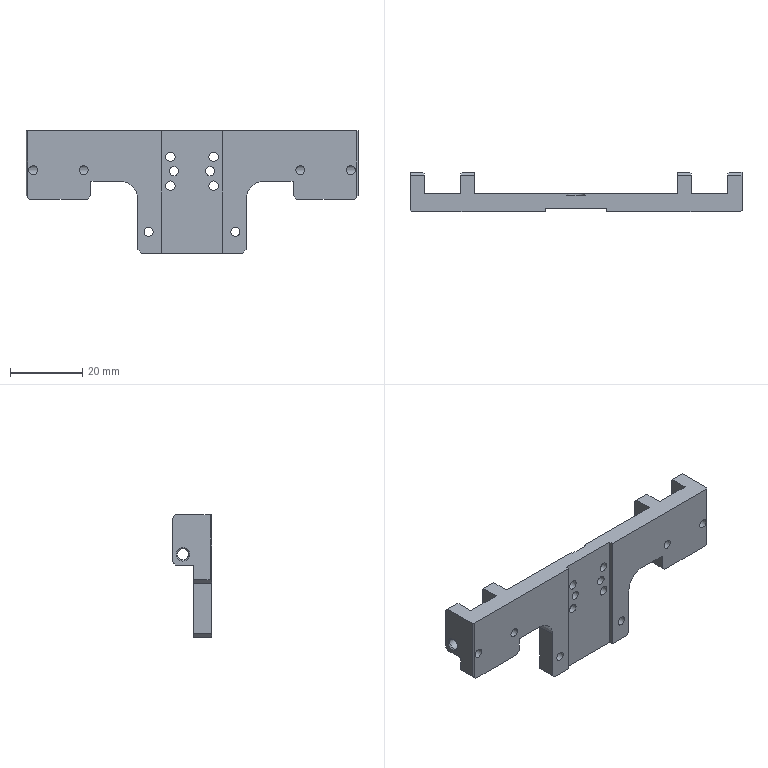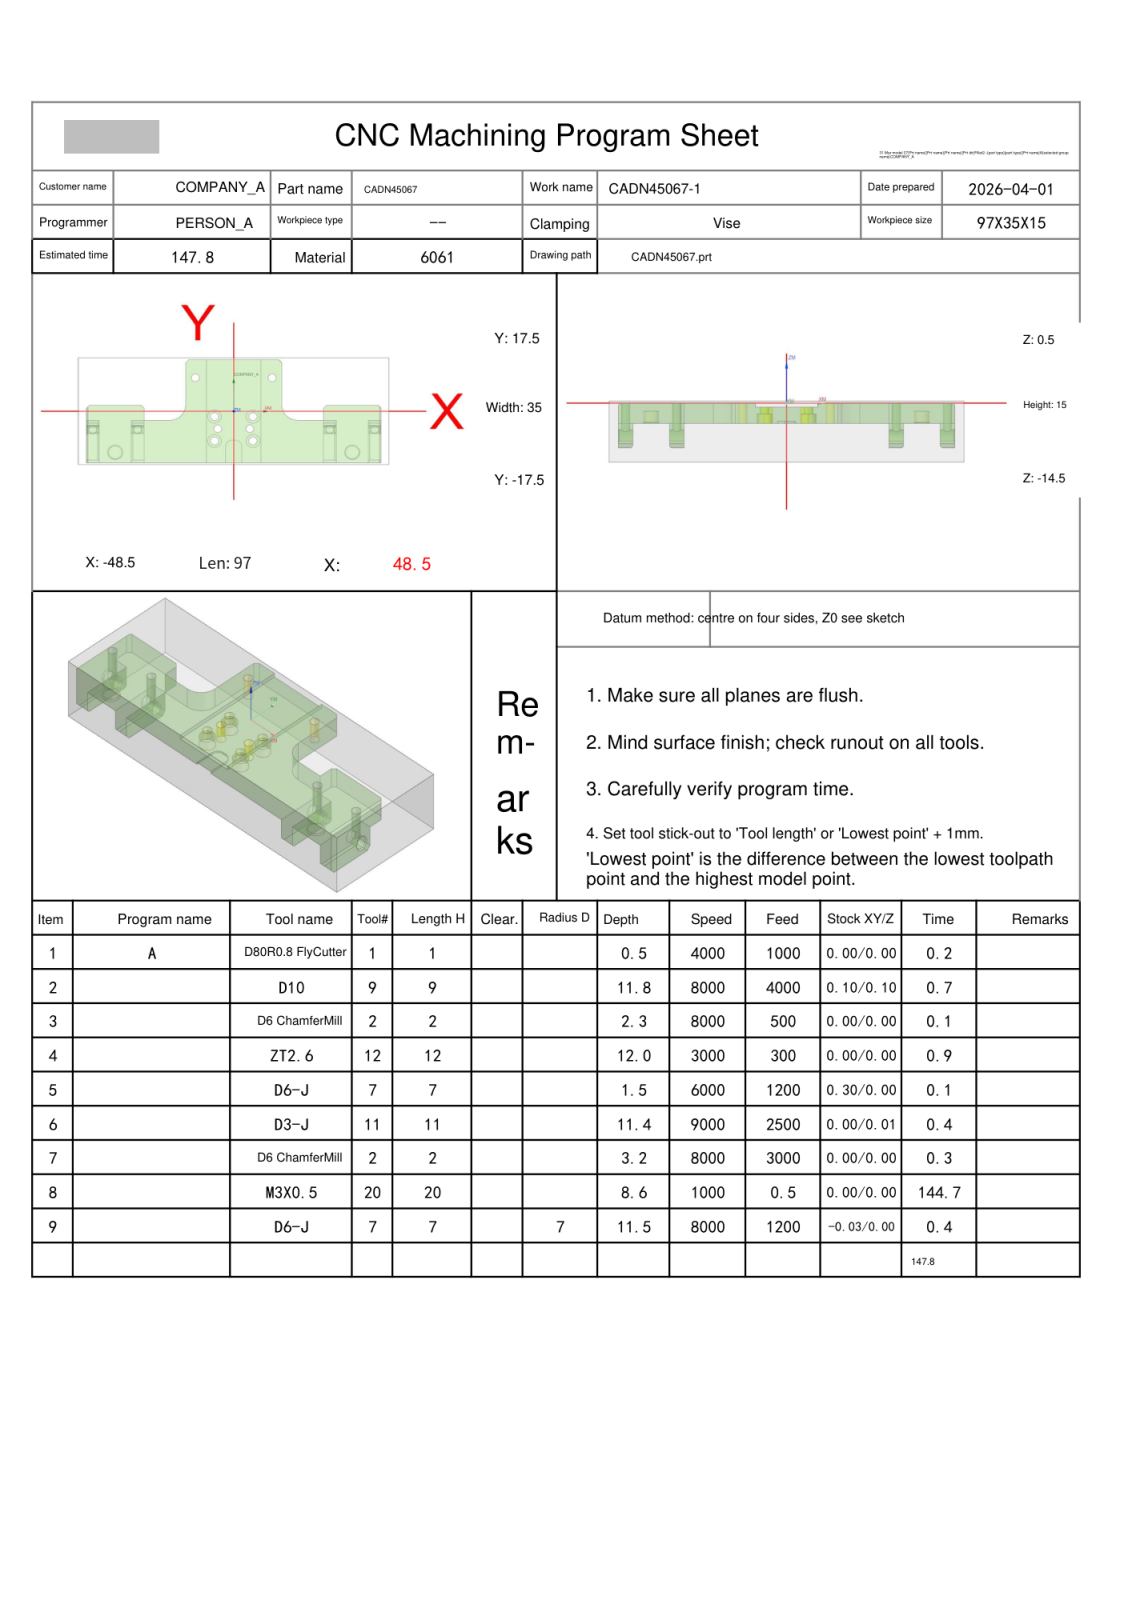NC program | NX | posted by the shop | part box 92 x 11 x 34 mm
Lines 1 to 973 of 3207:
%
O0001
(Machine time: 278.14 MIN)
(===Total Tool:7===)
(T1=D80R0.8 FlyCutter D=80.  R=0.8  D-  H01 Z=0.    )
(T9=D10     D=10.  R=0.   D-  H09 Z=-11.3 )
(T2=D6 ChamferMill   D=6.   R=0.   D-  H02 Z=-2.75 )
(T12=ZT2.6  D=2.6  DR_a=118 D-  H12 Z=-11.5 )
(T7=D6-J    D=6.   R=0.   D-  H07 Z=-11.  )
(T11=D3-J   D=3.   R=0.   D-  H11 Z=-10.95)
(T20=M3X0.5 D=2.5  DR_a=180 D-  H20 Z=-8.08 )
G80 G90 G17 G49 G40
G91 G28 Z0
M01
N1 T01 M06
(D80R0.8 FlyCutter  D=80. R=0.8 H=01 ce=0.00 di=0.00)
G00 G90 G54 X-91. Y0.0 M03 S4000
G43 H01 Z20.
M08
Z2.
G01 Z0.0 F1000.
X-86.
X86.
X91.
Z2.
G00 Z20.
G91 G28 Z0.0
M05
M09
G91 G28 Z0.0
M01
N2 T09 M06
(D10  D=10. R=0. H=09 ce=0.12 di=0.10)
G00 G90 G54 X-15.027 Y28.431 M03 S8000
G43 H09 Z20.
M08
Z-9.3
G01 X-15.008 Y28.332 Z-9.925 F4000.
X-14.99 Y28.234 Z-10.172
X-14.971 Y28.136 Z-10.354
X-14.952 Y28.038 Z-10.5
X-14.934 Y27.939 Z-10.623
X-14.915 Y27.841 Z-10.728
X-14.896 Y27.743 Z-10.82
X-14.877 Y27.645 Z-10.9
X-14.859 Y27.546 Z-10.97
X-14.84 Y27.448 Z-11.032
X-14.821 Y27.35 Z-11.086
X-14.803 Y27.252 Z-11.133
X-14.784 Y27.153 Z-11.174
X-14.765 Y27.055 Z-11.208
X-14.747 Y26.957 Z-11.236
X-14.728 Y26.859 Z-11.26
X-14.709 Y26.76 Z-11.277
X-14.691 Y26.662 Z-11.29
X-14.672 Y26.564 Z-11.297
X-14.653 Y26.466 Z-11.3
X-14.251 Y24.351
G03 X-13.992 Y24. I.505 J.101
X-10.185 Y23.362 I4.017 J12.298
X-.018 Y23.181 I10.167 J284.555
X3.308 Y23.2 I0.0 J284.737
G01 X46.748 Y23.176
G02 X52.525 Y19.311 I-.242 J-6.612
X53.961 Y13.361 I-14.623 J-6.679
X54.203 Y5.248 I-135.848 J-8.113
X54.195 Y3.766 I-136.09 J0.0
G01 X54.177 Y-15.734
G02 X50.311 Y-21.524 I-6.614 J.23
X44.597 Y-22.942 I-6.515 J14.043
X37.298 Y-23.208 I-7.299 J99.963
X35.644 Y-23.194 I0.0 J100.229
G01 X-46.67 Y-23.18
G02 X-52.525 Y-19.311 I.169 J6.619
X-53.961 Y-13.361 I14.611 J6.676
X-54.203 Y-5.248 I135.79 J8.112
X-54.195 Y-3.766 I136.032 J0.0
G01 X-54.176 Y15.75
G02 X-50.311 Y21.525 I6.611 J-.244
X-44.361 Y22.961 I6.676 J-14.611
X-36.248 Y23.203 I8.112 J-135.794
X-34.766 Y23.195 I0.0 J-136.036
G01 X-16.786 Y23.183
G03 X-9.6 Y22.58 I34.675 J369.909
X2.814 Y22.383 I12.414 J389.989
X6.589 Y22.401 I0.0 J390.187
G01 X44.649 Y22.383
G02 X51.148 Y18.321 I-.327 J-7.754
X52.998 Y12.151 I-13.989 J-7.555
X53.396 Y3.632 I-90.774 J-8.518
X53.388 Y2.404 I-91.173 J0.0
X53.417 Y-4.672 I-860.326 J-7.075
X53.368 Y-13.907 I-860.355 J0.0
X50.563 Y-19.305 I-7.563 J.502
X49.62 Y-20.62 I-7.355 J4.275
G01 X48.56 Y-21.434
X47.325 Y-21.946
G02 X42.258 Y-22.281 I-5.149 J39.324
X30.14 Y-22.402 I-12.117 J609.001
X28.179 Y-22.399 I0.0 J609.122
G01 X-44.667 Y-22.381
G02 X-46.751 Y-22.021 I.405 J8.572
G01 X-47.325 Y-21.946
X-48.56 Y-21.434
G02 X-51.669 Y-17.588 I4.721 J6.996
X-53.123 Y-11.141 I18.194 J7.492
X-53.415 Y-1.39 I162.948 J9.751
X-53.397 Y1.013 I163.239 J0.0
X-53.424 Y6.04 I476.588 J5.027
X-53.356 Y14.066 I476.615 J0.0
X-49.144 Y20.249 I7.789 J-.78
X-42.791 Y22.039 I7.593 J-14.778
X-34.291 Y22.397 I8.5 J-100.793
X-33.041 Y22.389 I0.0 J-101.151
X-27.007 Y22.413 I6.034 J-757.291
X-17.782 Y22.357 I0.0 J-757.315
G01 X-14. Y22.12
X14.002
G03 X21.353 Y21.621 I7.351 J53.976
X22.067 Y21.626 I0.0 J54.474
G01 X42.888 Y21.573
G02 X50.323 Y16.726 I-.459 J-8.829
X52.184 Y10.146 I-16.132 J-8.116
X52.592 Y1.241 I-97.093 J-8.905
X52.586 Y.159 I-97.5 J0.0
X52.62 Y-5.006 I-387.021 J-5.165
X52.554 Y-12.14 I-387.055 J0.0
X51.142 Y-16.521 I-10.912 J1.1
X50.946 Y-18.325 I-36.211 J3.033
G01 X50.486 Y-19.434
X50.946 Y-18.325
G03 X51.191 Y-16.06 I-107.777 J12.813
X51.934 Y-8.588 I-37.182 J7.472
X51.929 Y-7.943 I-37.925 J0.0
X51.975 Y-3.234 I-236.428 J4.709
X51.732 Y7.493 I-236.475 J0.0
X50.393 Y14.457 I-23.222 J-.855
X43.355 Y20.339 I-8.633 J-3.178
X36.831 Y20.923 I-6.524 J-36.141
X36.43 Y20.92 I0.0 J-36.725
G01 X20.998 Y21.011
G02 X16.923 Y21.209 I1.762 J77.998
G03 X15.325 Y21.946 I-4.315 J-7.262
G02 X17.068 Y21.098 I-2.104 J-6.544
G03 X21.136 Y20.363 I4.386 J12.641
X31.627 Y20.135 I10.491 J242.039
X33.802 Y20.145 I0.0 J242.266
G02 X34.726 Y20.153 I.924 J-52.036
X41.463 Y19.715 I0.0 J-52.044
X49.288 Y13.58 I-1.36 J-9.793
X50.86 Y6.421 I-21.035 J-8.371
X51.12 Y.998 I-168.616 J-10.807
G01 Y-16.602
G03 X51.62 Y-17.102 I.5 J0.0
X52.042 Y-16.87 I0.0 J.5
G01 X52.519 Y-16.12
X53.577 Y-14.456 Z-11.2
X53.787 Y-14.126
X53.82 Y-14.064
X53.845 Y-13.997
X53.86 Y-13.928
X53.865 Y-13.857
X53.843 Y-1.578
X53.835 Y-1.492
X53.813 Y-1.409
X53.777 Y-1.331
X53.728 Y-1.26
X53.668 Y-1.199
X53.601 Y-1.142
X52.102 Y.14 Z-11.3
X51.217 Y.904
X51.098 Y1.167
G03 X50.634 Y3.733 I-24.591 J-3.118
X49.669 Y9.816 I-82.833 J-10.024
X46.824 Y15.648 I-12.341 J-2.411
X40.893 Y18.792 I-7.983 J-7.892
X33.491 Y19.476 I-7.402 J-39.713
X33.175 Y19.475 I0.0 J-40.397
G01 X33.128
G02 X21.762 Y19.722 I0.0 J261.456
X17.923 Y20.349 I.585 J15.651
G01 X16.797 Y21.252
G02 X18.094 Y20.188 I-14.159 J-18.571
G03 X21.533 Y19.166 I4.228 J7.934
X29.648 Y18.728 I8.115 J74.925
G01 X29.936 Y18.729
G02 X30.535 Y18.731 I.599 J-69.867
X38.479 Y18.278 I0.0 J-69.87
X44.463 Y15.976 I-1.326 J-12.376
X48.465 Y9.807 I-7.838 J-9.468
X49.656 Y4.621 I-50.692 J-14.371
G03 X50.434 Y3.56 I34.496 J24.473
G01 X50.946 Y2.325
X50.434 Y3.56
G02 X48.775 Y6.744 I5.561 J4.922
G03 X46.649 Y11.993 I-23.04 J-6.278
X39.603 Y17.076 I-9.686 J-6.002
X32.394 Y17.988 I-7.697 J-31.896
G02 X23.157 Y18.396 I3.021 J172.774
X18.864 Y19.358 I.801 J13.637
G01 X17.943 Y20.298
G03 X19.127 Y19.093 I17.57 J16.084
X22.774 Y17.859 I4.705 J7.898
X30.924 Y17.248 I9.416 J70.916
G02 X38.38 Y16.381 I-.507 J-36.872
X46.34 Y9.984 I-2.75 J-11.572
X48.159 Y6.004 I-141.115 J-66.909
X49.67 Y4.556 I-10.941 J-12.928
G03 X47.965 Y6.178 I-18.761 J-18.016
G02 X46.018 Y9.28 I23.42 J16.86
G03 X37.168 Y15.73 I-11.564 J-6.569
X29.712 Y16.63 I-8.897 J-42.374
G02 X22.376 Y17.382 I1.532 J51.116
X19.525 Y18.434 I1.268 J7.822
G01 X18.752 Y19.449
G03 X19.762 Y18.136 I14.102 J9.803
X23.01 Y16.71 I4.642 J6.158
X30.29 Y15.811 I9.893 J50.186
G02 X37.459 Y14.642 I-1.63 J-32.559
X44.777 Y9.191 I-4.344 J-13.469
G03 X46.544 Y6.867 I20.238 J13.558
G01 X47.56 Y6.434
X48.195 Y5.947
G03 X46.523 Y6.863 I-2.961 J-3.418
G02 X44.818 Y8.41 I4.982 J7.206
G03 X40.12 Y12.463 I-15.238 J-12.914
X32.691 Y14.81 I-9.737 J-17.892
G02 X25.154 Y15.719 I67.012 J587.378
X20.504 Y17.158 I1.567 J13.289
X19.764 Y17.763 I1.305 J2.352
G01 X19.458 Y18.502
G03 X21.386 Y16.311 I3.259 J.923
X26.269 Y14.888 I6.975 J14.843
G02 X33.497 Y13.801 I-26.147 J-198.455
X43.023 Y8.857 I-3.33 J-18.065
G03 X45.107 Y7.123 I12.003 J12.304
G01 X46.325 Y6.946
X46.547 Y6.854
G03 X45.118 Y7.104 I-1.605 J-4.949
G02 X42.801 Y8.452 I2.84 J7.547
G03 X36.336 Y12.161 I-15.255 J-19.101
X29.481 Y13.736 I-11.603 J-34.788
G02 X23.173 Y15.042 I4.783 J39.005
X20.077 Y16.837 I1.902 J6.848
X19.946 Y17.325 I1.744 J.73
G01 X19.792 Y17.695
G02 X19.995 Y16.945 I-1.743 J-.874
G03 X21.615 Y15.273 I3.301 J1.575
X26.642 Y13.522 I7.797 J14.295
G02 X33.687 Y12.036 I-20.605 J-115.122
X40.856 Y8.697 I-6.729 J-23.815
G03 X43.531 Y7.136 I11.967 J17.443
G01 X45.16 Y7.099
G02 X43.26 Y7.157 I.25 J39.333
X40.456 Y8.363 I3.623 J12.289
G03 X29.687 Y12.224 I-17.114 J-30.783
G02 X23.482 Y13.837 I7.202 J40.426
X20.334 Y15.859 I2.442 J7.264
X20.083 Y16.282 I3.325 J2.265
G01 X19.989 Y16.996
G03 X21.201 Y14.646 I2.889 J.003
X25.609 Y12.505 I7.544 J9.926
X32.643 Y10.658 I247.224 J927.101
G02 X39.89 Y7.718 I-13.871 J-44.594
G03 X41.359 Y7.12 I21.725 J51.235
G01 X43.599
G02 X42.643 Y7.103 I-.956 J26.501
X40.78 Y7.168 I0.0 J26.518
X37.931 Y8.072 I3.982 J17.495
G03 X27.616 Y11.295 I-28.861 J-74.239
G02 X22.181 Y13.408 I4.812 J20.423
X20.152 Y15.386 I2.641 J4.739
G01 X20.089 Y16.236
G03 X20.172 Y15.174 I10.018 J.255
X22.207 Y12.875 I4.52 J1.951
X27.674 Y10.554 I10.734 J17.683
G02 X38.206 Y7.143 I-44.432 J-155.125
G01 X41.278 Y7.12
G02 X39.934 Y7.103 I-1.344 J54.929
X37.527 Y7.156 I0.0 J54.945
X33.621 Y8.13 I5.297 J29.554
X25.268 Y10.752 I30.263 J111.051
X20.984 Y13.335 I4.009 J11.494
X20.12 Y14.654 I2.195 J2.38
G01 Y15.454
G03 X20.098 Y15.061 I3.458 J-.392
X20.278 Y13.955 I3.48 J0.0
X22.904 Y11.298 I5.784 J3.09
X29.107 Y8.698 I14.082 J24.893
X34.374 Y7.12 I90.483 J292.457
G01 X37.974
G02 X36.278 Y7.099 I-1.695 J68.329
X33.182 Y7.169 I0.0 J68.35
X23.405 Y10.416 I4.91 J31.13
X20.353 Y13.126 I3.82 J7.374
X20.12 Y13.658 I4.083 J2.108
G01 Y14.618
G03 X20.099 Y14.157 I5.04 J-.461
X20.208 Y13.111 I5.061 J0.0
X22.528 Y10.379 I5.626 J2.426
X29.042 Y7.406 I12.619 J19.025
G01 X30.065 Y7.12
X33.825
X33.512
G02 X29.144 Y7.148 I0.0 J333.222
X21.39 Y10.748 I2.101 J14.675
X20.12 Y12.595 I2.906 J3.359
G01 Y13.555
G03 X20.097 Y13.079 I4.838 J-.476
X20.226 Y11.967 I4.861 J0.0
X22.675 Y9.098 I5.996 J2.637
X27.414 Y6.901 I8.436 J11.993
G02 X29.562 Y7.12 I2.16 J-10.567
G03 X29.32 Y7.124 I-.242 J-6.95
X27.478 Y6.876 I0.0 J-6.954
G02 X23.984 Y7.797 I.029 J7.191
X20.326 Y10.982 I3.542 J7.763
X20.12 Y11.478 I6.47 J2.973
G01 Y12.438
G03 X20.096 Y11.969 I4.612 J-.469
X20.257 Y10.758 I4.636 J0.0
X23.018 Y7.755 I6.089 J2.827
X26.485 Y6.478 I4.332 J6.418
G01 X27.635 Y6.929
G02 X26.248 Y6.415 I-2.98 J5.92
G01 X26.244
G02 X22.403 Y7.7 I0.0 J6.386
X20.128 Y10.331 I3.088 J4.97
G01 X20.12 Y11.333
G03 X20.096 Y10.865 I4.614 J-.469
X20.257 Y9.654 I4.638 J0.0
X23.673 Y6.467 I5.676 J2.661
X25.51 Y6.042 I1.837 J3.758
X25.907 Y6.061 I0.0 J4.183
G02 X26.588 Y6.495 I6.864 J-10.022
G03 X25.896 Y6.03 I2.483 J-4.439
G02 X24.968 Y5.919 I-.928 J3.827
X23.12 Y6.38 I0.0 J3.938
X20.134 Y9.228 I2.183 J5.279
G01 X20.12 Y10.274
G03 X20.095 Y9.805 I4.408 J-.469
X20.264 Y8.592 I4.433 J0.0
X25.035 Y5.553 I4.771 J2.225
G01 X25.138 Y5.554
G03 X25.983 Y6.084 I-.684 J2.031
G02 X24.925 Y5.451 I-1.725 J1.686
X24.467 Y5.429 I-.458 J4.612
X21.268 Y6.709 I0.0 J4.635
X20.12 Y8.314 I2.232 J2.809
G01 Y9.194
G03 X20.096 Y8.764 I3.816 J-.43
X20.272 Y7.614 I3.84 J0.0
X24.259 Y5.086 I3.987 J1.88
X24.728 Y5.111 I0.0 J4.408
X25.381 Y5.621 I-.493 J1.304
G02 X23.954 Y4.897 I-1.427 J1.043
X23.64 Y4.925 I0.0 J1.767
X20.136 Y7.341 I.343 J4.247
G01 X20.12 Y8.312
G03 X20.098 Y7.883 I4.169 J-.429
X20.217 Y6.889 I4.191 J0.0
X23.713 Y4.614 I3.496 J1.548
X24.333 Y4.664 I0.0 J3.823
X24.987 Y5.227 I-1.016 J1.842
G02 X24.223 Y4.58 I-1.922 J1.493
X23.347 Y4.467 I-.876 J3.346
X20.942 Y5.44 I0.0 J3.458
X20.12 Y6.634 I1.547 J1.945
G01 Y7.274
G03 X20.098 Y6.941 I2.48 J-.334
X21.383 Y4.754 I2.502 J0.0
X23.197 Y4.156 I1.815 J2.454
X24.054 Y4.279 I0.0 J3.052
X24.494 Y4.735 I-6.713 J6.919
G02 X23.91 Y4.169 I-1.68 J1.15
X22.956 Y4.019 I-.955 J2.958
X20.544 Y5.167 I0.0 J3.109
X20.099 Y6.231 I1.053 J1.065
X20.12 Y6.48 I1.497 J0.0
G03 X20.1 Y6.182 I2.174 J-.299
X21.207 Y4.275 I2.195 J0.0
X22.881 Y3.729 I1.674 J2.292
X23.718 Y3.855 I0.0 J2.838
X24.172 Y4.354 I-1.535 J1.854
G02 X22.815 Y3.559 I-1.357 J.761
X22.523 Y3.587 I0.0 J1.556
X20.131 Y5.21 I.157 J2.805
G01 X20.12 Y5.911
G03 X20.097 Y5.588 I2.199 J-.322
X20.34 Y4.577 I2.223 J0.0
X22.58 Y3.326 I2.24 J1.379
X23.446 Y3.473 I0.0 J2.63
G01 X23.862 Y3.956
G02 X22.559 Y3.166 I-1.303 J.678
X22.329 Y3.184 I0.0 J1.469
X20.14 Y4.602 I.117 J2.58
G01 X20.12 Y5.266
G03 X20.099 Y4.98 I1.905 J-.286
X21.399 Y3.158 I1.926 J0.0
X22.341 Y2.93 I.941 J1.826
X23.37 Y3.206 I0.0 J2.055
X23.606 Y3.627 I-3.777 J2.388
G02 X22.502 Y2.811 I-1.103 J.338
G01 X22.451 Y2.812
G02 X22.248 Y2.804 I-.203 J2.37
X20.141 Y4.079 I0.0 J2.378
G01 X20.12 Y4.665
G03 X20.104 Y4.428 I1.721 J-.237
X21.267 Y2.789 I1.737 J0.0
X22.173 Y2.562 I.905 J1.696
X23.243 Y2.888 I0.0 J1.922
G01 X23.493 Y3.373
G02 X22.321 Y2.45 I-1.172 J.283
G01 X22.288 Y2.451
G02 X22.052 Y2.438 I-.235 J2.119
X20.135 Y3.638 I0.0 J2.132
G01 X20.12 Y4.127
G03 X20.106 Y3.916 I1.55 J-.211
X21.093 Y2.462 I1.565 J0.0
X22.028 Y2.212 I.935 J1.623
X23.094 Y2.545 I0.0 J1.873
G01 X23.34 Y3.025
G02 X22.289 Y2.12 I-1.132 J.252
X21.97 Y2.095 I-.319 J2.054
X20.146 Y3.178 I0.0 J2.079
G01 X20.12 Y3.699
G03 X20.1 Y3.465 I1.372 J-.234
X21.133 Y2.12 I1.392 J0.0
G01 X21.853
G02 X21.512 Y2.098 I-.341 J2.665
X20.779 Y2.2 I0.0 J2.687
X20.113 Y3.149 I.343 J.948
G01 X20.12 Y3.264
G03 X20.099 Y3.06 I.971 J-.204
X20.773 Y2.12 I.992 J0.0
G01 X21.093
X20.909 Y2.099
G02 X20.189 Y2.511 I0.0 J.836
X20.126 Y2.766 I.487 J.255
X20.676 Y3.316 I.55 J0.0
X21.086 Y3.133 I0.0 J-.55
X21.301 Y2.682 I-.365 J-.451
X21.129 Y2.269 I-.581 J0.0
X20.756 Y2.126 I-.373 J.414
G01 X20.651 Y2.136
G02 X20.107 Y2.763 I.091 J.627
G01 X20.12 Y2.889
X20.115 Y2.802
G03 X20.298 Y2.298 I.782 J0.0
X20.729 Y2.12 I.486 J.565
X21.45 Y2.101 I.721 J13.948
X22.744 Y2.161 I0.0 J13.966
X23.217 Y2.921 I-.373 J.759
G01 X23.213 Y2.995
X22.514 Y5.899
X22.501 Y6.015
G02 X22.627 Y6.352 I.512 J0.0
G01 X22.693 Y6.427 Z-11.297
X22.759 Y6.501 Z-11.29
X22.825 Y6.576 Z-11.277
X22.892 Y6.651 Z-11.26
X22.958 Y6.726 Z-11.236
X23.024 Y6.801 Z-11.208
X23.09 Y6.876 Z-11.174
X23.157 Y6.951 Z-11.133
X23.223 Y7.026 Z-11.086
X23.289 Y7.101 Z-11.032
X23.355 Y7.176 Z-10.97
X23.422 Y7.251 Z-10.9
X23.488 Y7.326 Z-10.82
X23.554 Y7.401 Z-10.728
X23.62 Y7.475 Z-10.623
X23.687 Y7.55 Z-10.5
X23.753 Y7.625 Z-10.354
X23.819 Y7.7 Z-10.172
X23.885 Y7.775 Z-9.925
X23.951 Y7.85 Z-9.3
G00 Z20.
X45.893 Y-26.117
Z-9.3
G01 X45.95 Y-26.034 Z-9.925
X46.006 Y-25.952 Z-10.172
X46.063 Y-25.87 Z-10.354
X46.12 Y-25.787 Z-10.5
X46.177 Y-25.705 Z-10.623
X46.233 Y-25.623 Z-10.728
X46.29 Y-25.54 Z-10.82
X46.347 Y-25.458 Z-10.9
X46.404 Y-25.376 Z-10.97
X46.461 Y-25.294 Z-11.032
X46.517 Y-25.211 Z-11.086
X46.574 Y-25.129 Z-11.133
X46.631 Y-25.047 Z-11.174
X46.688 Y-24.964 Z-11.208
X46.745 Y-24.882 Z-11.236
X46.801 Y-24.8 Z-11.26
X46.858 Y-24.717 Z-11.277
X46.915 Y-24.635 Z-11.29
X46.972 Y-24.553 Z-11.297
X47.028 Y-24.47 Z-11.3
G03 X47.117 Y-24.183 I-.423 J.288
G01 X47.083 Y-23.998
X46.468 Y-22.44
G03 X45.998 Y-22.12 I-.472 J-.188
G01 X-46.002
X-47.325 Y-21.946
X-48.56 Y-21.434
X-49.62 Y-20.62
X-50.434 Y-19.56
G02 X-51.31 Y-16.737 I9.725 J4.566
X-52.522 Y-5.625 I50.944 J11.178
X-52.619 Y4.221 I500.143 J9.846
X-52.557 Y12.113 I500.24 J0.0
X-47.741 Y19.313 I8.799 J-.674
X-41.082 Y21.191 I8.148 J-16.151
X-32.022 Y21.596 I9.06 J-101.264
X-30.774 Y21.588 I0.0 J-101.669
X-26.234 Y21.617 I4.54 J-348.163
X-17.835 Y21.516 I0.0 J-348.193
G03 X-16.902 Y21.471 I.933 J9.569
X-16.445 Y21.482 I0.0 J9.614
G01 X-15.325 Y21.946
X-14.056 Y22.113
X-15.325 Y21.946
G02 X-18.891 Y21.108 I-3.566 J7.171
G01 X-18.901
G02 X-29.059 Y20.932 I-10.158 J293.951
X-31.323 Y20.941 I0.0 J294.126
G03 X-32.407 Y20.948 I-1.084 J-78.317
X-41.303 Y20.442 I0.0 J-78.325
X-47.4 Y18.396 I1.629 J-14.963
X-51.309 Y12.474 I5.056 J-7.588
X-51.921 Y5.872 I35.291 J-6.602
X-51.918 Y5.392 I35.903 J0.0
X-51.966 Y.923 I207.889 J-4.469
X-51.725 Y-9.084 I207.937 J0.0
X-51.12 Y-14.117 I57.333 J4.338
G01 Y-16.998
X-50.946 Y-18.325
X-51.12 Y-16.998
X-51.098 Y5.321
G02 X-51.1 Y5.653 I28.242 J.331
X-50.433 Y11.752 I28.244 J0.0
X-44.727 Y18.221 I9.444 J-2.579
X-37.502 Y19.853 I8.441 J-20.561
X-26.986 Y20.176 I10.516 J-171.02
X-25.208 Y20.167 I0.0 J-171.343
G03 X-24.144 Y20.157 I1.064 J56.509
X-18.166 Y20.474 I0.0 J56.519
X-17.619 Y20.621 I-1.127 J5.274
G01 X-16.56 Y21.434
G02 X-18.024 Y20.389 I-5.679 J6.407
X-22.104 Y19.689 I-4.34 J13.054
X-33.304 Y19.418 I-16.653 J457.415
G03 X-41.319 Y18.521 I.284 J-38.764
X-47.197 Y15.256 I2.408 J-11.26
X-49.928 Y9.19 I9.232 J-7.805
X-50.444 Y3.535 I48.03 J-7.232
G01 X-50.946 Y2.325
X-51.12 Y1.002
X-50.946 Y2.325
G03 X-49.695 Y6.239 I-13.38 J6.432
G02 X-48.216 Y11.502 I21.69 J-3.254
X-41.817 Y17.088 I9.91 J-4.896
X-34.131 Y18.488 I8.693 J-25.92
X-23.694 Y18.836 I24.177 J-568.765
G03 X-18.765 Y19.545 I-.199 J18.873
X-17.619 Y20.621 I-4.223 J5.641
G02 X-19.01 Y19.345 I-5.849 J4.976
X-22.801 Y18.4 I-4.481 J9.901
X-31.788 Y17.954 I-12.14 J154.021
G03 X-39.858 Y16.878 I.615 J-35.41
X-46.551 Y12.22 I2.8 J-11.16
X-48.722 Y6.995 I15.351 J-9.443
G02 X-49.418 Y4.823 I-10.942 J2.307
G03 X-50.434 Y3.56 I13.762 J-12.114
G02 X-49.066 Y5.253 I39.478 J-30.492
G03 X-47.426 Y8.666 I-27.066 J15.106
G02 X-39.109 Y15.893 I11.72 J-5.089
X-31.061 Y17.117 I9.151 J-33.109
G03 X-23.059 Y17.639 I-4.566 J131.587
X-19.42 Y18.603 I-.841 J10.518
G01 X-18.619 Y19.622
G02 X-19.62 Y18.401 I-5.944 J3.855
X-22.905 Y17.212 I-4.352 J6.89
X-30.405 Y16.516 I-10.233 J69.437
G03 X-38.373 Y15.291 I1.323 J-35.139
X-46.378 Y8.752 I3.768 J-12.781
G02 X-47.831 Y6.226 I-102.211 J57.134
G03 X-49.355 Y4.886 I5.179 J-7.424
G02 X-47.415 Y6.567 I10.745 J-10.439
G03 X-44.996 Y9.494 I-37.945 J33.817
G02 X-36.28 Y14.744 I12.032 J-10.117
X-29.238 Y15.745 I10.026 J-45.268
G03 X-22.466 Y16.614 I-2.399 J45.479
X-19.821 Y17.735 I-1.484 J7.182
X-19.385 Y18.623 I-6.892 J3.934
G01 X-19.785 Y17.736
G02 X-22.166 Y16.317 I-3.695 J3.492
X-27.894 Y15.271 I-7.888 J26.986
G03 X-35.71 Y14.117 I4.392 J-56.794
X-44.65 Y8.627 I3.915 J-16.399
G02 X-46.259 Y6.972 I-11.553 J9.623
G01 X-47.56 Y6.434
G03 X-45.571 Y7.302 I-4.958 J14.076
X-42.073 Y10. I-77.11 J103.578
G02 X-32.804 Y13.731 I12.553 J-17.806
X-25.59 Y14.79 I101.297 J-665.078
G03 X-20.936 Y16.234 I-1.87 J14.251
X-20.012 Y16.999 I-1.092 J2.258
G02 X-19.731 Y17.843 I4.016 J-.87
G03 X-20.005 Y16.954 I2.358 J-1.213
G02 X-22.049 Y15.345 I-3.542 J2.398
X-27.425 Y13.941 I-8.11 J20.052
G03 X-34.878 Y12.532 I8.872 J-67.366
X-42.56 Y8.674 I6.146 J-21.814
G02 X-44.888 Y7.138 I-11.15 J14.374
G01 X-46.267 Y6.953
G03 X-44.307 Y7.243 I-1.241 J15.178
X-40.795 Y9.022 I-9.041 J22.202
G02 X-30.628 Y12.535 I15.221 J-27.582
G03 X-24.001 Y13.932 I-10.288 J65.225
X-20.497 Y15.731 I-2.225 J8.647
X-20.081 Y16.298 I-1.026 J1.189
G01 X-19.976 Y17.091
G02 X-20.175 Y16.005 I-3.339 J.049
X-22.432 Y14.119 I-4.217 J2.752
X-27.878 Y12.46 I-9.465 J21.297
G03 X-35.759 Y10.487 I10.394 J-58.264
X-41.914 Y7.666 I19.789 J-51.293
G02 X-43.252 Y7.12 I-10.438 J23.692
G01 X-44.932
G03 X-44.113 Y7.099 I.819 J16.211
X-42.4 Y7.19 I0.0 J16.231
X-38.17 Y8.686 I-7.433 J27.739
G02 X-30.13 Y11.119 I18.89 J-47.921
G03 X-23.69 Y12.866 I-8.95 J45.738
X-20.463 Y14.92 I-2.677 J7.769
X-20.1 Y15.786 I-.852 J.866
X-20.12 Y16.002 I-1.215 J0.0
G01 X-20.088 Y16.24
X-20.129 Y15.369
G02 X-21.839 Y13.402 I-3.76 J1.541
X-26.682 Y11.378 I-8.809 J14.273
G03 X-34.656 Y9.209 I44.655 J-179.886
G01 X-40.53 Y7.138
X-42.947 Y7.12
G03 X-41.768 Y7.099 I1.18 J33.226
X-39.376 Y7.185 I0.0 J33.247
X-34.061 Y8.575 I-10.278 J50.175
X-25.773 Y10.876 I-63.002 J242.963
X-21.139 Y13.262 I-3.696 J12.87
X-20.133 Y14.553 I-2.367 J2.883
G01 X-20.12 Y15.517
G02 X-20.101 Y15.117 I-4.243 J-.4
X-20.186 Y14.272 I-4.261 J0.0
X-22.351 Y11.955 I-4.75 J2.27
X-27.948 Y9.635 I-11.158 J19.006
X-36.949 Y7.12 I-173.546 J603.728
G01 X-40.069
G03 X-38.275 Y7.095 I1.794 J65.466
X-35.242 Y7.166 I0.0 J65.491
X-24.305 Y10.181 I-6.841 J46.148
X-20.548 Y12.839 I-3.685 J9.194
X-20.12 Y13.624 I-1.552 J1.356
G01 Y14.584
G02 X-20.101 Y14.154 I-4.977 J-.43
X-20.183 Y13.255 I-4.996 J0.0
X-22.264 Y10.857 I-4.984 J2.223
X-28.022 Y8.254 I-11.378 J17.497
X-32.246 Y7.12 I-21.116 J70.231
G01 X-35.846
G03 X-34.036 Y7.108 I1.811 J139.291
X-30.485 Y7.153 I0.0 J139.303
X-22.053 Y10.29 I-2.125 J18.613
X-20.135 Y12.449 I-3.257 J4.823
G01 X-20.12 Y13.58
G02 X-20.1 Y13.115 I-5.594 J-.465
X-20.18 Y12.172 I-5.614 J0.0
X-22.309 Y9.647 I-5.23 J2.249
X-28.355 Y7.035 I-9.566 J13.837
G03 X-30.174 Y7.142 I-1.819 J-15.46
X-30.998 Y7.12 I0.0 J-15.567
G02 X-30.171 Y7.14 I.828 J-17.365
X-27.857 Y6.985 I0.0 J-17.385
G03 X-20.625 Y10.52 I-.556 J10.303
X-20.12 Y11.42 I-1.923 J1.672
G01 Y12.54
G02 X-20.099 Y12.041 I-5.944 J-.499
X-20.183 Y11.046 I-5.965 J0.0
X-22.436 Y8.421 I-5.283 J2.255
X-26.953 Y6.67 I-5.624 J7.806
G03 X-28.071 Y6.998 I-1.694 J-3.714
G02 X-26.914 Y6.633 I-.306 J-2.991
G03 X-26.143 Y6.579 I.771 J5.477
X-23.678 Y7.159 I0.0 J5.531
X-20.164 Y10.132 I-2.574 J6.604
X-20.097 Y10.901 I-4.364 J.768
X-20.12 Y11.351 I-4.431 J0.0
G02 X-20.101 Y10.891 I-5.594 J-.46
X-20.182 Y9.941 I-5.612 J0.0
X-22.518 Y7.345 I-4.948 J2.103
X-26.08 Y6.247 I-3.64 J5.482
G01 X-27.031 Y6.679
G02 X-26.183 Y6.244 I-.709 J-2.425
G03 X-25.054 Y6.079 I1.129 J3.785
X-23.521 Y6.389 I0.0 J3.949
X-20.157 Y9.097 I-1.828 J5.714
X-20.109 Y9.914 I-6.942 J.817
X-20.12 Y10.303 I-6.99 J0.0
G02 X-20.101 Y9.838 I-5.651 J-.464
X-20.179 Y8.899 I-5.67 J0.0
X-22.817 Y6.307 I-4.523 J1.966
X-24.882 Y5.791 I-2.064 J3.869
X-25.664 Y5.861 I0.0 J4.385
G01 X-26.26 Y6.296
G03 X-24.465 Y5.547 I1.795 J1.777
X-23.854 Y5.622 I0.0 J2.526
X-20.14 Y8.17 I-.689 J4.985
G01 X-20.12 Y9.235
G02 X-20.1 Y8.804 I-4.669 J-.43
X-20.186 Y7.911 I-4.688 J0.0
X-23.331 Y5.415 I-4.077 J1.906
X-24.242 Y5.288 I-.91 J3.2
X-25.134 Y5.41 I0.0 J3.327
G01 X-25.696 Y5.863
G03 X-24.947 Y5.274 I5.114 J5.735
X-23.773 Y5.083 I1.174 J3.519
X-21.857 Y5.616 I0.0 J3.71
X-20.128 Y7.341 I-1.452 J3.184
G01 X-20.12 Y8.268
G02 X-20.1 Y7.871 I-3.919 J-.397
X-20.191 Y7.03 I-3.939 J0.0
X-23.711 Y4.83 I-3.521 J1.717
X-24.634 Y4.94 I0.0 J3.917
X-25.191 Y5.432 I1.726 J2.517
G03 X-23.467 Y4.578 I1.724 J1.313
X-23.034 Y4.622 I0.0 J2.167
X-20.154 Y6.452 I-.389 J3.793
X-20.12 Y7.298 I-10.427 J.846
G01 Y7.333
G02 X-20.1 Y6.992 I-2.942 J-.341
X-20.197 Y6.243 I-2.962 J0.0
X-23.238 Y4.364 I-3.042 J1.523
X-24.254 Y4.519 I0.0 J3.402
G01 X-24.775 Y5.015
G03 X-23.749 Y4.242 I1.848 J1.385
X-22.987 Y4.154 I.762 J3.221
X-20.153 Y5.753 I0.0 J3.31
X-20.12 Y6.537 I-14.736 J1.006
G02 X-20.095 Y6.224 I-1.964 J-.314
X-20.302 Y5.341 I-1.989 J0.0
X-22.851 Y3.927 I-2.549 J1.591
X-23.982 Y4.148 I0.0 J3.005
G01 X-24.365 Y4.601
G03 X-22.793 Y3.698 I1.571 J.915
X-22.473 Y3.726 I0.0 J1.818
X-20.15 Y5.13 I-.163 J2.894
G01 X-20.12 Y5.827
G02 X-20.098 Y5.552 I-1.736 J-.275
X-21.059 Y3.985 I-1.757 J0.0
X-22.579 Y3.506 I-1.52 J2.173
X-23.661 Y3.737 I0.0 J2.652
G01 X-24.045 Y4.192
G03 X-22.452 Y3.285 I1.593 J.945
X-21.966 Y3.35 I0.0 J1.853
X-20.155 Y4.547 I-.388 J2.555
G01 X-20.12 Y5.189
G02 X-20.099 Y4.937 I-1.531 J-.252
X-20.916 Y3.571 I-1.551 J0.0
X-22.327 Y3.111 I-1.411 J1.934
X-23.428 Y3.379 I0.0 J2.394
G01 X-23.704 Y3.754
G03 X-22.371 Y2.923 I1.332 J.653
G01 X-22.296 Y2.925
X-22.128 Y2.919
G03 X-20.141 Y4.086 I0.0 J2.275
G01 X-20.12 Y4.672
G02 X-20.099 Y4.424 I-1.446 J-.248
X-20.939 Y3.097 I-1.468 J0.0
X-22.13 Y2.736 I-1.191 J1.784
X-23.338 Y3.109 I0.0 J2.145
G01 X-23.565 Y3.536
G03 X-22.238 Y2.559 I1.327 J.412
G01 X-22.156 Y2.561
G03 X-21.95 Y2.551 I.206 J2.054
X-20.141 Y3.62 I0.0 J2.065
G01 X-20.12 Y4.126
G02 X-20.102 Y3.911 I-1.285 J-.215
X-20.807 Y2.754 I-1.303 J0.0
X-21.987 Y2.379 I-1.18 J1.666
X-23.204 Y2.781 I0.0 J2.042
G01 X-23.405 Y3.173
G03 X-22.096 Y2.207 I1.309 J.404
G01 X-22.029 Y2.208
G03 X-21.825 Y2.198 I.204 J1.922
X-20.144 Y3.175 I0.0 J1.933
G01 X-20.12 Y3.692
X-20.107 Y3.506
G02 X-21.006 Y2.248 I-1.33 J0.0
X-21.841 Y2.098 I-.835 J2.257
X-22.996 Y2.393 I0.0 J2.406
G01 X-23.05 Y2.452
G02 X-23.198 Y2.827 I.403 J.375
X-22.774 Y3.362 I.55 J0.0
G01 X-20.707 Y3.841
X-20.671 Y3.842
G02 X-20.12 Y3.292 I0.0 J-.551
X-21.302 Y2.116 I-1.182 J.006
G01 X-21.397 Y2.12
G03 X-21.175 Y2.098 I.222 J1.091
X-20.12 Y2.856 I0.0 J1.113
G01 Y3.176
X-20.097 Y2.979
G02 X-20.963 Y2.113 I-.866 J0.0
G01 X-21.074 Y2.12
X-20.884 Y2.097
G03 X-20.214 Y2.454 I0.0 J.807
X-20.128 Y2.749 I-.466 J.295
X-20.68 Y3.3 I-.551 J0.0
X-21.231 Y2.749 I0.0 J-.551
G01 X-21.229 Y2.709
X-21.23 Y2.691
G03 X-20.679 Y2.141 I.55 J0.0
G01 X-20.572 Y2.151
G03 X-20.108 Y2.766 I-.175 J.615
G01 X-20.12 Y2.889
X-20.115 Y2.802
G02 X-20.298 Y2.298 I-.782 J0.0
X-20.729 Y2.12 I-.486 J.565
X-21.451 Y2.101 I-.722 J13.878
X-22.744 Y2.162 I0.0 J13.897
X-23.247 Y2.816 I.467 J.879
G01 X-23.283 Y2.934
X-23.289 Y3.057
X-23.017 Y6.744
X-23.01 Y6.843 Z-11.297
X-23.003 Y6.943 Z-11.29
X-22.995 Y7.043 Z-11.277
X-22.988 Y7.143 Z-11.26
X-22.981 Y7.242 Z-11.236
X-22.973 Y7.342 Z-11.208
X-22.966 Y7.442 Z-11.174
X-22.959 Y7.541 Z-11.133
X-22.951 Y7.641 Z-11.086
X-22.944 Y7.741 Z-11.032
X-22.937 Y7.841 Z-10.97
X-22.929 Y7.94 Z-10.9
X-22.922 Y8.04 Z-10.82
X-22.915 Y8.14 Z-10.728
X-22.907 Y8.24 Z-10.623
X-22.9 Y8.339 Z-10.5
X-22.893 Y8.439 Z-10.354
X-22.885 Y8.539 Z-10.172
X-22.878 Y8.638 Z-9.925
X-22.871 Y8.738 Z-9.3
G00 Z20.
G00 G90 X0.0 Y-25. M03 S6000
Z20.
Z.05
G01 Z-.45 F3500.
Y-18.
X3.4
Y18.
X-3.4
Y-18.
X0.0
X.5
Z.05
G00 Z.5
X0.0 Y-25.
Z-.4
G01 Z-.9
Y-18.
X3.4
Y18.
X-3.4
Y-18.
X0.0
X.5
Z-.4
G00 Z20.
G91 G28 Z0.0
M05
M09
G91 G28 Z0.0
M01
N3 T02 M06
(D6 ChamferMill  D=6. R=0. H=02 ce=0.00 di=0.10)
G00 G90 G54 X-44. Y-6. M03 S8000
G43 H02 Z20.
M08
G98 G81 X-44. Y-6. Z-.8 R1. F500.
X-30.
X-12. Y11.
X-6. Y-1.75 Z-1.8 R0.0
X-5. Y-5.75
X-6. Y-9.75
X6.
X5. Y-5.75
X6. Y-1.75
X12. Y11. Z-.8 R1.
X30. Y-6.
X44.
G80
G00 Z20.
G91 G28 Z0.0
M05
M09
G91 G28 Z0.0
M01
N4 T12 M06
(ZT2.6 D=2.6 DR_a=118 H=12)
G00 G90 G54 X6. Y-1.75 M03 S3000
G43 H12 Z20.
M08
G98 G83 X6. Y-1.75 Z-5.481 R0.0 F80. Q2.5
Y-9.75
X-6.
Y-1.75
G80
G00 Z20.
G00 G90 X12. Y11. M03 S3000
Z20.
G98 G83 X12. Y11. Z-10.5 R1. F300. Q2.
X5. Y-5.75 Z-11.5 R0.0
X-5.
X-12. Y11. Z-10.5 R1.
G80
G00 Z20.
G00 G90 X-44. Y-6. M03 S3000
Z20.
G98 G83 X-44. Y-6. Z-8.8 R1. F100. Q2.
X-30.
X30.
X44.
G80
G00 Z20.
G91 G28 Z0.0
M05
M09
G91 G28 Z0.0
M01
N5 T07 M06
(D6-J  D=6. R=0. H=07 ce=0.30 di=0.00)
G00 G90 G54 X0.0 Y-23. M03 S6000
G43 H07 Z20.
M08
Z-.5
G01 Z-1. F1200.
Y-17.6
X-5.2
Y17.6
X5.2
Y-17.6
X0.0
Y-13.4
X-1.
Y13.4
X1.
Y-13.4
X0.0
X-.5
Y-23.
Z-.5
G00 Z20.
G91 G28 Z0.0
M05
M09
G91 G28 Z0.0
M01